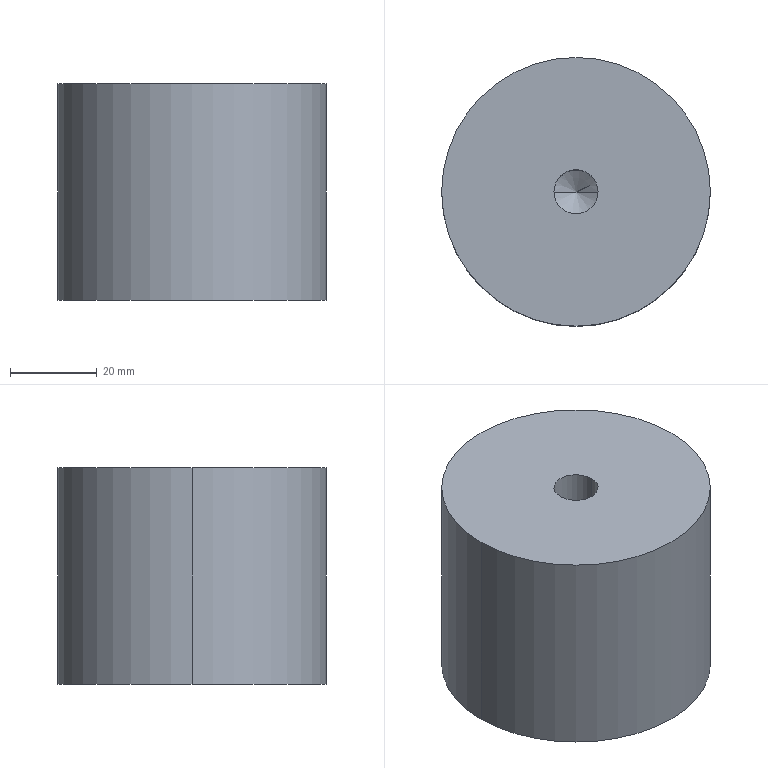Part | SolidWorks | features Extrusion 1, HoleWzd 1 | 1 solid | 8 faces | box 62 x 62 x 50 mm | volume 148480 mm3 | cylinder 4 | cone 2 | plane 2 | commonest cylinder face diameters 10.2 x2 62 x2
STEP:
#1=CARTESIAN_POINT('',(-5.1,0.,20.75));
#2=VERTEX_POINT('',#1);
#3=CARTESIAN_POINT('',(5.1,0.,20.75));
#4=VERTEX_POINT('',#3);
#5=CARTESIAN_POINT('',(0.,0.,20.75));
#6=DIRECTION('',(0.,0.,1.));
#7=DIRECTION('',(1.,0.,0.));
#8=AXIS2_PLACEMENT_3D('',#5,#6,#7);
#9=CIRCLE('',#8,5.1);
#10=EDGE_CURVE('',#2,#4,#9,.T.);
#11=ORIENTED_EDGE('',*,*,#10,.F.);
#12=CARTESIAN_POINT('',(-5.1,0.,50.));
#13=VERTEX_POINT('',#12);
#14=CARTESIAN_POINT('',(-5.1,0.,50.));
#15=DIRECTION('',(0.,0.,1.));
#16=VECTOR('',#15,1000.);
#17=LINE('',#14,#16);
#18=EDGE_CURVE('',#2,#13,#17,.T.);
#19=ORIENTED_EDGE('',*,*,#18,.T.);
#20=CARTESIAN_POINT('',(5.1,0.,50.));
#21=VERTEX_POINT('',#20);
#22=CARTESIAN_POINT('',(0.,0.,50.));
#23=DIRECTION('',(0.,0.,1.));
#24=DIRECTION('',(1.,0.,0.));
#25=AXIS2_PLACEMENT_3D('',#22,#23,#24);
#26=CIRCLE('',#25,5.1);
#27=EDGE_CURVE('',#13,#21,#26,.T.);
#28=ORIENTED_EDGE('',*,*,#27,.T.);
#29=CARTESIAN_POINT('',(5.1,0.,50.));
#30=DIRECTION('',(0.,0.,1.));
#31=VECTOR('',#30,1000.);
#32=LINE('',#29,#31);
#33=EDGE_CURVE('',#4,#21,#32,.T.);
#34=ORIENTED_EDGE('',*,*,#33,.F.);
#35=EDGE_LOOP('',(#11,#19,#28,#34));
#36=FACE_OUTER_BOUND('',#35,.T.);
#37=CARTESIAN_POINT('',(0.,0.,50.));
#38=DIRECTION('',(0.,0.,1.));
#39=DIRECTION('',(1.,0.,0.));
#40=AXIS2_PLACEMENT_3D('',#37,#38,#39);
#41=CYLINDRICAL_SURFACE('',#40,5.1);
#42=ADVANCED_FACE('',(#36),#41,.F.);
#43=CARTESIAN_POINT('',(0.,0.,17.686));
#44=VERTEX_POINT('',#43);
#45=CARTESIAN_POINT('',(5.1,0.,20.75));
#46=DIRECTION('',(0.8572,0.,0.515));
#47=VECTOR('',#46,1000.);
#48=LINE('',#45,#47);
#49=EDGE_CURVE('',#44,#4,#48,.T.);
#50=ORIENTED_EDGE('',*,*,#49,.F.);
#51=CARTESIAN_POINT('',(-5.1,0.,20.75));
#52=DIRECTION('',(-0.8572,0.,0.515));
#53=VECTOR('',#52,1000.);
#54=LINE('',#51,#53);
#55=EDGE_CURVE('',#44,#2,#54,.T.);
#56=ORIENTED_EDGE('',*,*,#55,.T.);
#57=ORIENTED_EDGE('',*,*,#10,.T.);
#58=EDGE_LOOP('',(#50,#56,#57));
#59=FACE_OUTER_BOUND('',#58,.T.);
#60=CARTESIAN_POINT('',(0.,0.,20.75));
#61=DIRECTION('',(0.,0.,1.));
#62=DIRECTION('',(1.,0.,0.));
#63=AXIS2_PLACEMENT_3D('',#60,#61,#62);
#64=CONICAL_SURFACE('',#63,5.1,1.03);
#65=ADVANCED_FACE('',(#59),#64,.F.);
#66=CARTESIAN_POINT('',(31.,0.,50.));
#67=VERTEX_POINT('',#66);
#68=CARTESIAN_POINT('',(-31.,0.,50.));
#69=VERTEX_POINT('',#68);
#70=CARTESIAN_POINT('',(0.,0.,50.));
#71=DIRECTION('',(0.,0.,1.));
#72=DIRECTION('',(1.,0.,0.));
#73=AXIS2_PLACEMENT_3D('',#70,#71,#72);
#74=CIRCLE('',#73,31.);
#75=EDGE_CURVE('',#67,#69,#74,.T.);
#76=ORIENTED_EDGE('',*,*,#75,.F.);
#77=CARTESIAN_POINT('',(31.,0.,0.));
#78=VERTEX_POINT('',#77);
#79=CARTESIAN_POINT('',(31.,0.,50.));
#80=DIRECTION('',(0.,0.,-1.));
#81=VECTOR('',#80,1000.);
#82=LINE('',#79,#81);
#83=EDGE_CURVE('',#67,#78,#82,.T.);
#84=ORIENTED_EDGE('',*,*,#83,.T.);
#85=CARTESIAN_POINT('',(-31.,0.,0.));
#86=VERTEX_POINT('',#85);
#87=CARTESIAN_POINT('',(0.,0.,0.));
#88=DIRECTION('',(0.,0.,1.));
#89=DIRECTION('',(1.,0.,0.));
#90=AXIS2_PLACEMENT_3D('',#87,#88,#89);
#91=CIRCLE('',#90,31.);
#92=EDGE_CURVE('',#78,#86,#91,.T.);
#93=ORIENTED_EDGE('',*,*,#92,.T.);
#94=CARTESIAN_POINT('',(-31.,0.,50.));
#95=DIRECTION('',(0.,0.,-1.));
#96=VECTOR('',#95,1000.);
#97=LINE('',#94,#96);
#98=EDGE_CURVE('',#69,#86,#97,.T.);
#99=ORIENTED_EDGE('',*,*,#98,.F.);
#100=EDGE_LOOP('',(#76,#84,#93,#99));
#101=FACE_OUTER_BOUND('',#100,.T.);
#102=CARTESIAN_POINT('',(0.,0.,50.));
#103=DIRECTION('',(0.,0.,-1.));
#104=DIRECTION('',(-1.,0.,0.));
#105=AXIS2_PLACEMENT_3D('',#102,#103,#104);
#106=CYLINDRICAL_SURFACE('',#105,31.);
#107=ADVANCED_FACE('',(#101),#106,.T.);
#108=ORIENTED_EDGE('',*,*,#83,.F.);
#109=CARTESIAN_POINT('',(0.,0.,50.));
#110=DIRECTION('',(0.,0.,1.));
#111=DIRECTION('',(1.,0.,0.));
#112=AXIS2_PLACEMENT_3D('',#109,#110,#111);
#113=CIRCLE('',#112,31.);
#114=EDGE_CURVE('',#69,#67,#113,.T.);
#115=ORIENTED_EDGE('',*,*,#114,.F.);
#116=ORIENTED_EDGE('',*,*,#98,.T.);
#117=CARTESIAN_POINT('',(0.,0.,0.));
#118=DIRECTION('',(0.,0.,1.));
#119=DIRECTION('',(1.,0.,0.));
#120=AXIS2_PLACEMENT_3D('',#117,#118,#119);
#121=CIRCLE('',#120,31.);
#122=EDGE_CURVE('',#86,#78,#121,.T.);
#123=ORIENTED_EDGE('',*,*,#122,.T.);
#124=EDGE_LOOP('',(#108,#115,#116,#123));
#125=FACE_OUTER_BOUND('',#124,.T.);
#126=CARTESIAN_POINT('',(0.,0.,50.));
#127=DIRECTION('',(0.,0.,-1.));
#128=DIRECTION('',(-1.,0.,0.));
#129=AXIS2_PLACEMENT_3D('',#126,#127,#128);
#130=CYLINDRICAL_SURFACE('',#129,31.);
#131=ADVANCED_FACE('',(#125),#130,.T.);
#132=CARTESIAN_POINT('',(0.,0.,50.));
#133=DIRECTION('',(0.,0.,1.));
#134=DIRECTION('',(1.,0.,0.));
#135=AXIS2_PLACEMENT_3D('',#132,#133,#134);
#136=CIRCLE('',#135,5.1);
#137=EDGE_CURVE('',#21,#13,#136,.T.);
#138=ORIENTED_EDGE('',*,*,#137,.F.);
#139=ORIENTED_EDGE('',*,*,#27,.F.);
#140=EDGE_LOOP('',(#138,#139));
#141=FACE_BOUND('',#140,.T.);
#142=ORIENTED_EDGE('',*,*,#114,.T.);
#143=ORIENTED_EDGE('',*,*,#75,.T.);
#144=EDGE_LOOP('',(#142,#143));
#145=FACE_OUTER_BOUND('',#144,.T.);
#146=CARTESIAN_POINT('',(0.,0.,50.));
#147=DIRECTION('',(0.,0.,1.));
#148=DIRECTION('',(1.,0.,0.));
#149=AXIS2_PLACEMENT_3D('',#146,#147,#148);
#150=PLANE('',#149);
#151=ADVANCED_FACE('',(#141,#145),#150,.T.);
#152=ORIENTED_EDGE('',*,*,#122,.F.);
#153=ORIENTED_EDGE('',*,*,#92,.F.);
#154=EDGE_LOOP('',(#152,#153));
#155=FACE_OUTER_BOUND('',#154,.T.);
#156=CARTESIAN_POINT('',(0.,0.,0.));
#157=DIRECTION('',(0.,0.,1.));
#158=DIRECTION('',(1.,0.,0.));
#159=AXIS2_PLACEMENT_3D('',#156,#157,#158);
#160=PLANE('',#159);
#161=ADVANCED_FACE('',(#155),#160,.F.);
#162=ORIENTED_EDGE('',*,*,#55,.F.);
#163=ORIENTED_EDGE('',*,*,#49,.T.);
#164=CARTESIAN_POINT('',(0.,0.,20.75));
#165=DIRECTION('',(0.,0.,1.));
#166=DIRECTION('',(1.,0.,0.));
#167=AXIS2_PLACEMENT_3D('',#164,#165,#166);
#168=CIRCLE('',#167,5.1);
#169=EDGE_CURVE('',#4,#2,#168,.T.);
#170=ORIENTED_EDGE('',*,*,#169,.T.);
#171=EDGE_LOOP('',(#162,#163,#170));
#172=FACE_OUTER_BOUND('',#171,.T.);
#173=CARTESIAN_POINT('',(0.,0.,20.75));
#174=DIRECTION('',(0.,0.,1.));
#175=DIRECTION('',(1.,0.,0.));
#176=AXIS2_PLACEMENT_3D('',#173,#174,#175);
#177=CONICAL_SURFACE('',#176,5.1,1.03);
#178=ADVANCED_FACE('',(#172),#177,.F.);
#179=ORIENTED_EDGE('',*,*,#18,.F.);
#180=ORIENTED_EDGE('',*,*,#169,.F.);
#181=ORIENTED_EDGE('',*,*,#33,.T.);
#182=ORIENTED_EDGE('',*,*,#137,.T.);
#183=EDGE_LOOP('',(#179,#180,#181,#182));
#184=FACE_OUTER_BOUND('',#183,.T.);
#185=CARTESIAN_POINT('',(0.,0.,50.));
#186=DIRECTION('',(0.,0.,1.));
#187=DIRECTION('',(1.,0.,0.));
#188=AXIS2_PLACEMENT_3D('',#185,#186,#187);
#189=CYLINDRICAL_SURFACE('',#188,5.1);
#190=ADVANCED_FACE('',(#184),#189,.F.);
#191=CLOSED_SHELL('',(#42,#65,#107,#131,#151,#161,#178,#190));
#192=MANIFOLD_SOLID_BREP('',#191);
#193=CARTESIAN_POINT('',(0.,0.,0.));
#194=DIRECTION('',(0.,0.,1.));
#195=DIRECTION('',(1.,0.,0.));
#196=AXIS2_PLACEMENT_3D('',#193,#194,#195);
#197=(LENGTH_UNIT()NAMED_UNIT(*)SI_UNIT(.MILLI.,.METRE.));
#198=UNCERTAINTY_MEASURE_WITH_UNIT(LENGTH_MEASURE(0.00001),#197,'','');
#199=(NAMED_UNIT(*)PLANE_ANGLE_UNIT()SI_UNIT($,.RADIAN.));
#200=(NAMED_UNIT(*)SI_UNIT($,.STERADIAN.)SOLID_ANGLE_UNIT());
#201=(GEOMETRIC_REPRESENTATION_CONTEXT(3)GLOBAL_UNCERTAINTY_ASSIGNED_CONTEXT((#198))GLOBAL_UNIT_ASSIGNED_CONTEXT((#197,#199,#200))REPRESENTATION_CONTEXT('',''));
#202=ADVANCED_BREP_SHAPE_REPRESENTATION('',(#192,#196),#201);